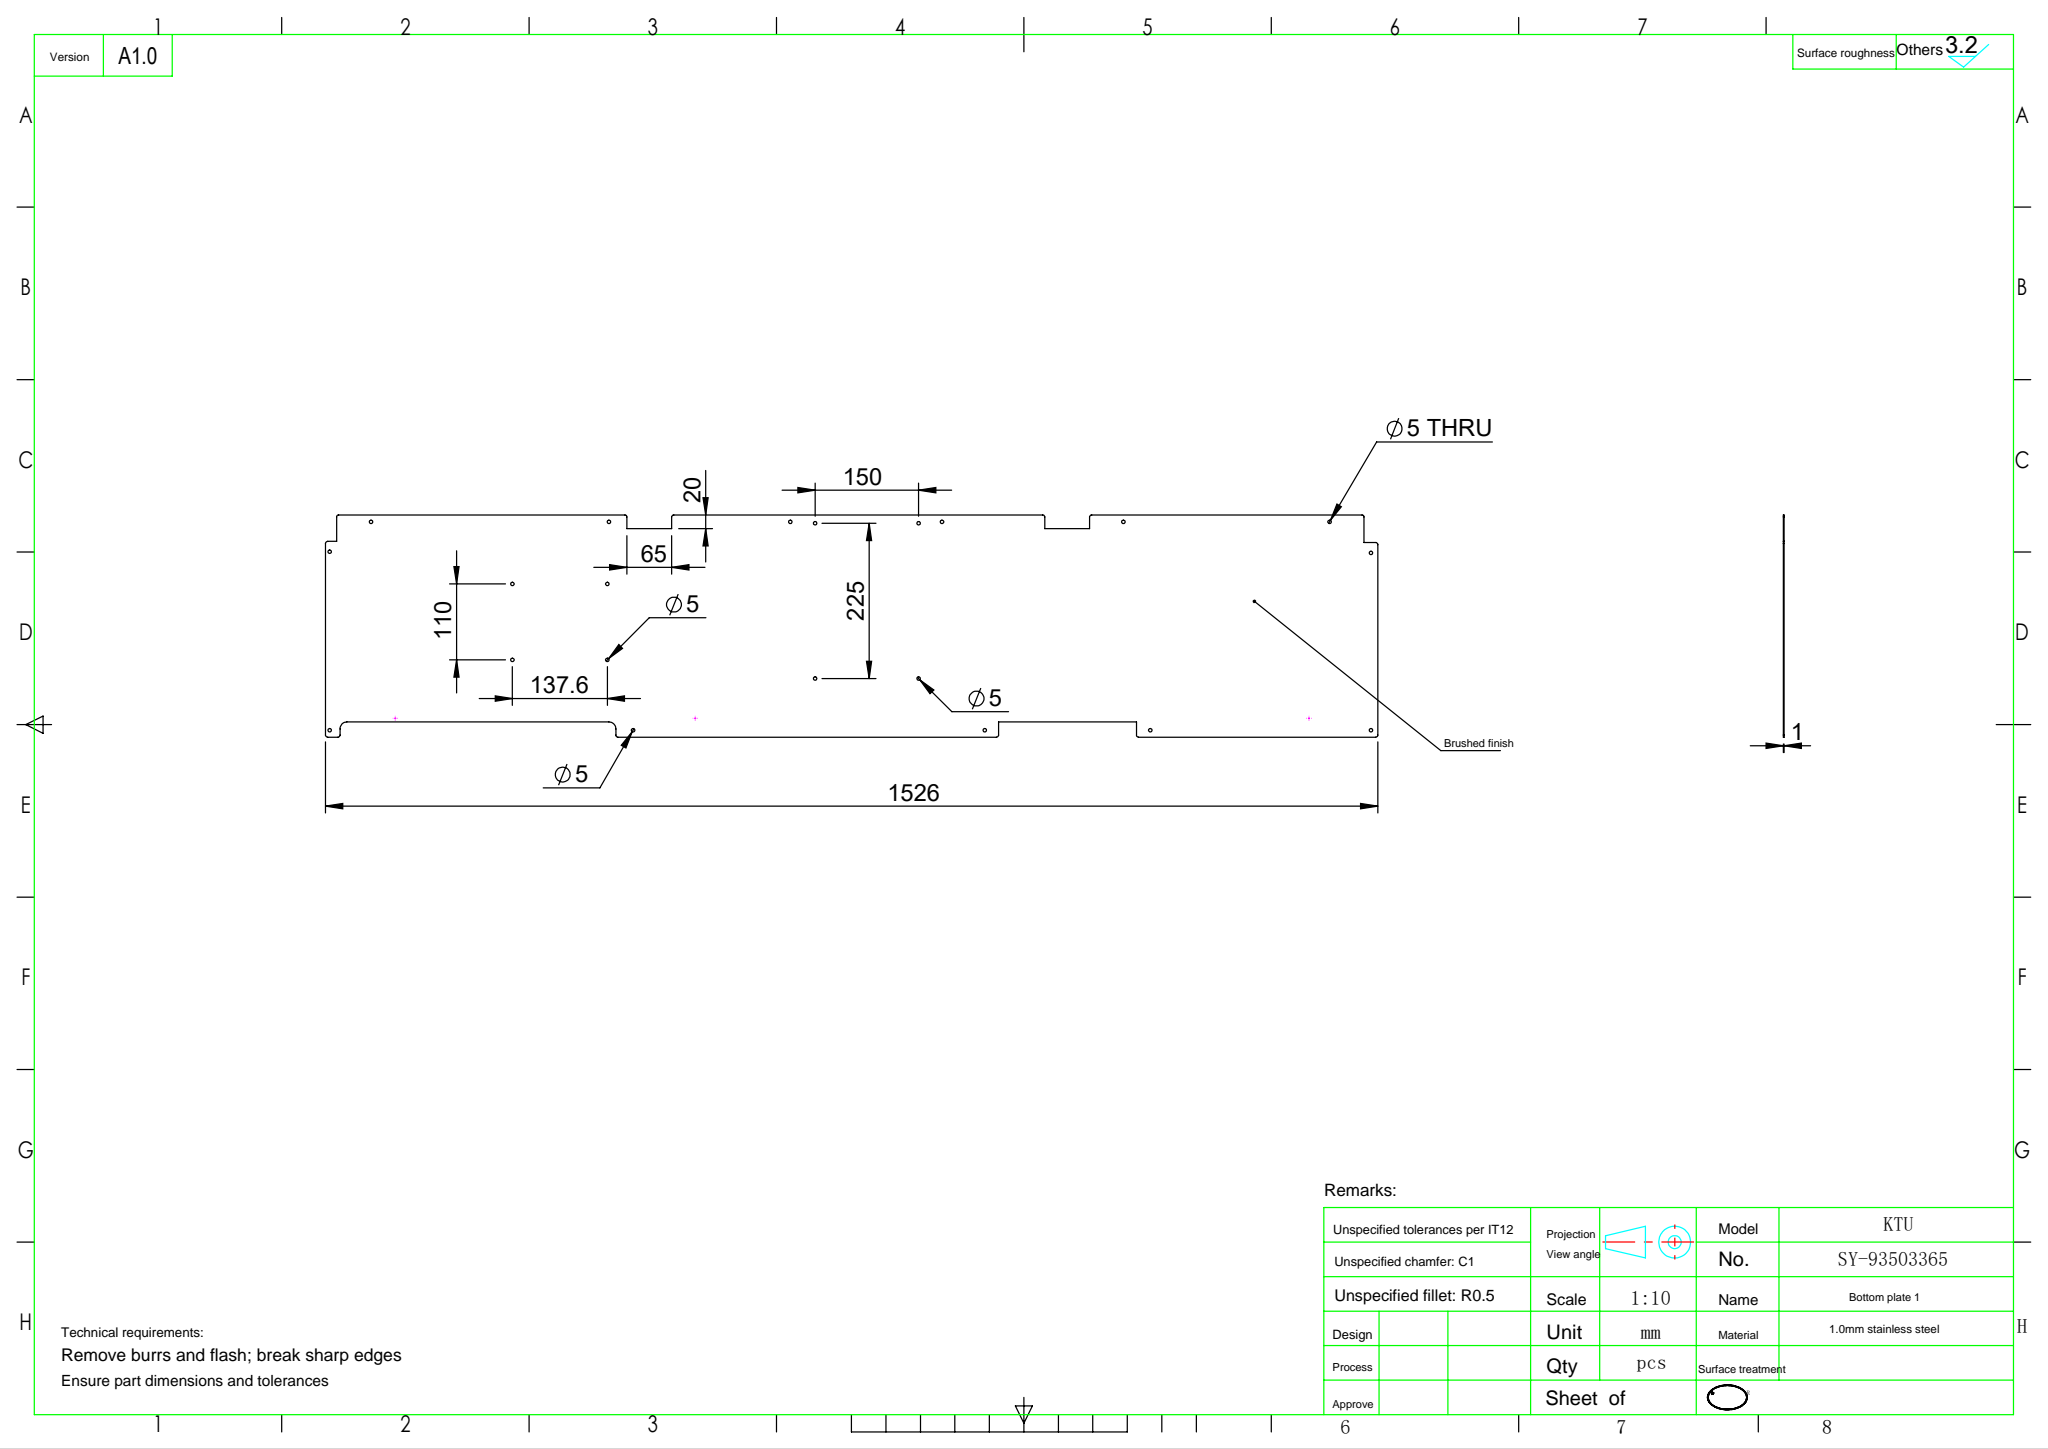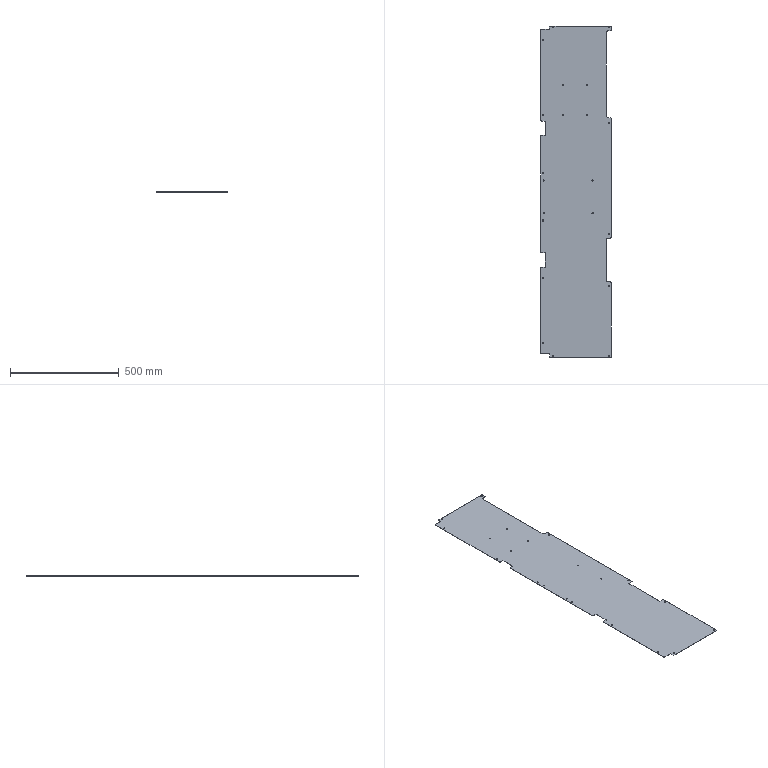Part | SolidWorks | features ICE 7, Fillet 5, Cut 3, FlatPattern 1, SMBaseFlange 1, SheetMetal 1 | 1 solid | 84 faces | box 322 x 1526 x 1 mm | volume 473763 mm3 | cylinder 58 | plane 26 | commonest cylinder face diameters 5 x42 6 x14 20 x2